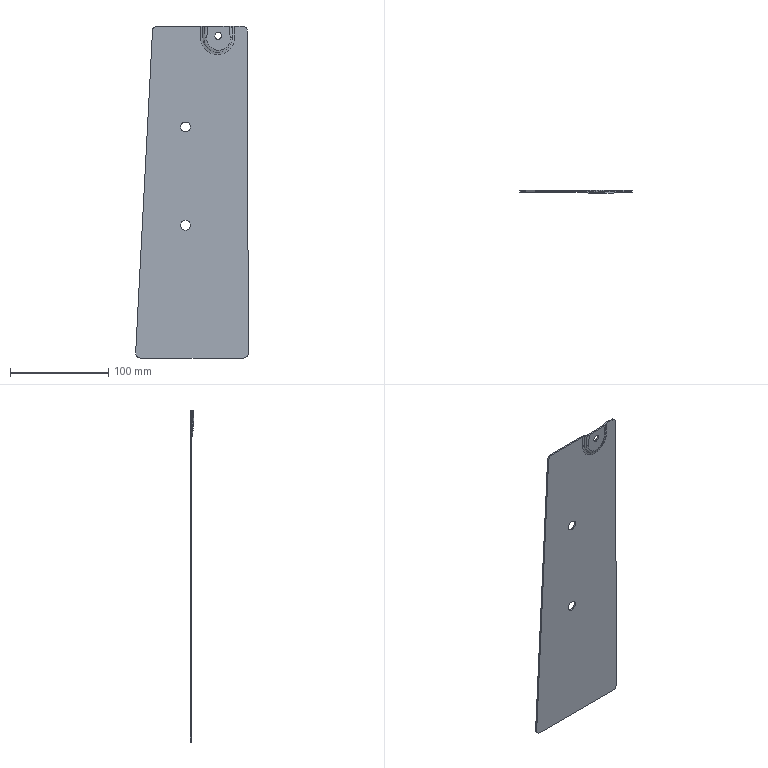Part | 1 solid | 48 faces | box 114.636 x 4.054 x 337.656 mm | volume 53110 mm3 | spline 25 | cylinder 14 | plane 5 | other 4 | commonest cylinder face diameters 10 x8 7 x4 13 x2